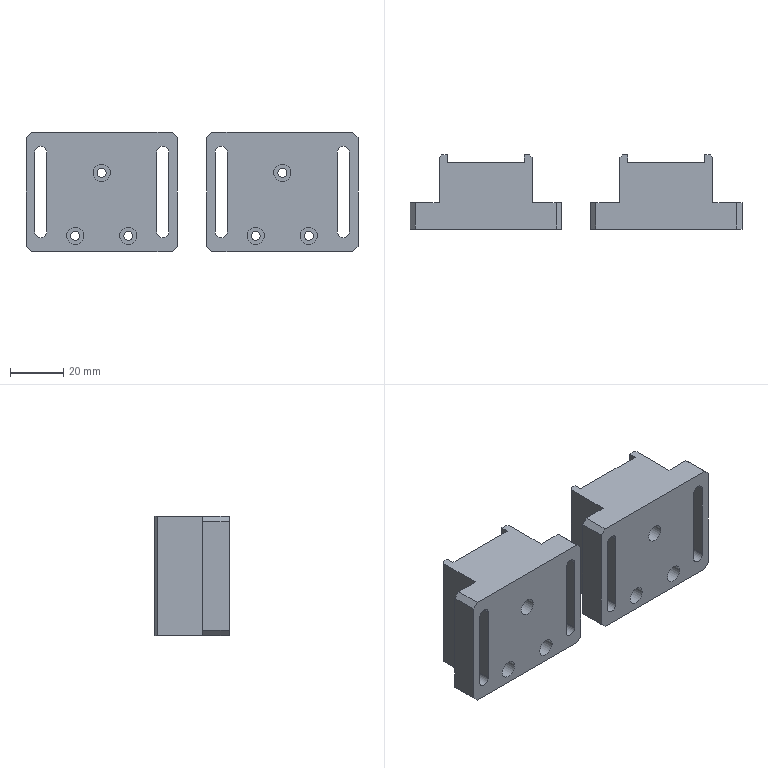CAM job | NX | 3+2 milling, drilling | part box 125 x 28 x 45 mm | stock box 129 x 30 x 50 mm
Tools:
number,name,description,diameter,corner_radius,flute_length,length,flutes
4,D4,平底铣刀-粗,4.0,0.0,25.0,75.0,2
9,D10,平底铣刀-粗,10.0,0.0,35.0,75.0,2
17,D4-J,平底铣刀-精,4.0,0.0,50.0,75.0,2
10,D10-J,平底铣刀-精,10.0,0.0,35.0,75.0,2
1,D80R0.8飞刀,圆鼻刀-粗,80.0,0.8,50.0,75.0,2
1,D80R0.8飞刀-J,圆鼻刀-精,80.0,0.8,50.0,75.0,2
2,D6倒角刀,倒角刀,6.0,0.0,3.0,25.0,2
13,ZT3.4,钻头,3.4,0.0,35.0,50.0,2
Operations:
program,operation,operation_type,tool,method,geometry_group,spindle_rpm,surface_speed,feed_per_tooth,feed_cut,feed_plunge,cut_length_mm,path_length_mm,cut_time_min,machine_time_min
B,底壁铣飞面一刀开粗_COPY,VolumeBased25DMillingOperation,D80R0.8飞刀,分层开粗-切深K-步距G,W-B,5000.0,1256.637,0.3,3000.0,100.0,932.776,1654.735,0.3109,0.3831
B,底壁铣飞面一刀精光_COPY,VolumeBased25DMillingOperation,D80R0.8飞刀-J,侧刃精光-切深K-步距G,W-B,5000.0,1256.637,0.1,1000.0,100.0,232.998,268.998,0.233,0.2366
B,底壁铣分层开粗-中_COPY,VolumeBased25DMillingOperation,D10,分层开粗-切深K-步距G,W-B,8000.0,251.327,0.25,4000.0,100.0,21759.4,22097.052,5.44,5.474
B,底壁铣分层开粗-中_COPY_1,VolumeBased25DMillingOperation,D10,分层开粗-切深K-步距G,W-B,8000.0,251.32,0.25,4000.0,100.0,2544.96,2650.146,0.6362,0.6468
B,钻倒角_1,Operation,D6倒角刀,METHOD,W-B,8000.0,150.796,0.0625,1000.0,0.0,30.0,261.337,0.03,0.0531
B,底壁铣倒角_COPY,VolumeBased25DMillingOperation,D6倒角刀,爬面_倒角-切深0-步距G,W-B,6500.0,122.519,0.1154,1500.0,100.0,215.202,481.218,0.1435,0.1701
B,平面去毛刺6X45L_COPY,SurfaceContour,D6倒角刀,爬面_倒角-切深0-步距G,W-B,6500.0,122.519,0.1154,1500.0,100.0,1059.156,2466.155,0.7061,0.8468
B,底壁铣精光底面-中_COPY_1,VolumeBased25DMillingOperation,D10-J,精光步距切深关,W-B,8000.0,251.32,0.0625,1000.0,100.0,606.44,721.888,0.6064,0.618
B,底壁铣精光底面-中_COPY,VolumeBased25DMillingOperation,D10-J,精光步距切深关,W-B,8000.0,251.32,0.0625,1000.0,100.0,714.094,990.365,0.7141,0.7417
B,底壁铣精光侧面-中-选底面_COPY,VolumeBased25DMillingOperation,D10-J,侧刃精光-切深K-步距G,W-B,8000.0,251.32,0.0625,1000.0,100.0,509.455,896.085,0.5095,0.5481
B,底壁铣精光侧面-中-选底面_COPY_1,VolumeBased25DMillingOperation,D10-J,侧刃精光-切深K-步距G,W-B,8000.0,251.32,0.0625,1000.0,100.0,252.2,373.086,0.2522,0.2643
A,顶面,FaceMilling,D80R0.8飞刀,侧刃精光-切深K-步距G,W-A,4000.0,1005.31,0.125,1000.0,100.0,219.0,255.0,0.219,0.2226
A,外形粗_2,VolumeBased25DMillingOperation,D10,METHOD,W-A,8000.0,251.327,0.3125,5000.0,80.0,27303.299,27503.799,5.461,5.481
A,沉头孔打点-深0.8,Operation,D6倒角刀,NONE,W-A,8000.0,150.796,0.0312,500.0,90.0,25.2,534.39,0.0504,0.1013
A,沉头孔-钻孔0段,Operation,ZT3.4,NONE,W-A,2800.0,29.908,0.0536,300.0,90.0,286.3,1032.482,0.9543,1.029
A,通腰槽粗_1,VolumeBased25DMillingOperation,D4,METHOD,W-A,6000.0,75.398,0.2083,2500.0,100.0,11219.504,11529.215,4.488,4.519
A,铣孔开粗D4_1,CylinderMilling,D4,NONE,W-A,8000.0,100.531,0.125,2000.0,100.0,3030.105,3526.552,1.515,1.565
A,铣孔精光D4_1,CylinderMilling,D4-J,精光步距切深关,W-A,8000.0,100.531,0.0375,600.0,100.0,299.202,795.648,0.4987,0.5483
A,腰槽精_1,VolumeBased25DMillingOperation,D4-J,METHOD,W-A,6000.0,113.0,0.0833,1000.0,100.0,765.589,1190.807,0.7656,0.8081
A,仅选体,SurfaceContour,D6倒角刀,METHOD,W-A,8000.0,150.796,0.1875,3000.0,100.0,733.671,1158.576,0.2446,0.287
A,铣倒角_1,PlanarMilling,D6倒角刀,NONE,W-A,8000.0,150.796,0.0312,500.0,100.0,175.533,534.535,0.3511,0.387
A,外形半精_2,VolumeBased25DMillingOperation,D10-J,METHOD,W-A,8000.0,251.327,0.0625,1000.0,100.0,1424.756,2081.215,1.425,1.49